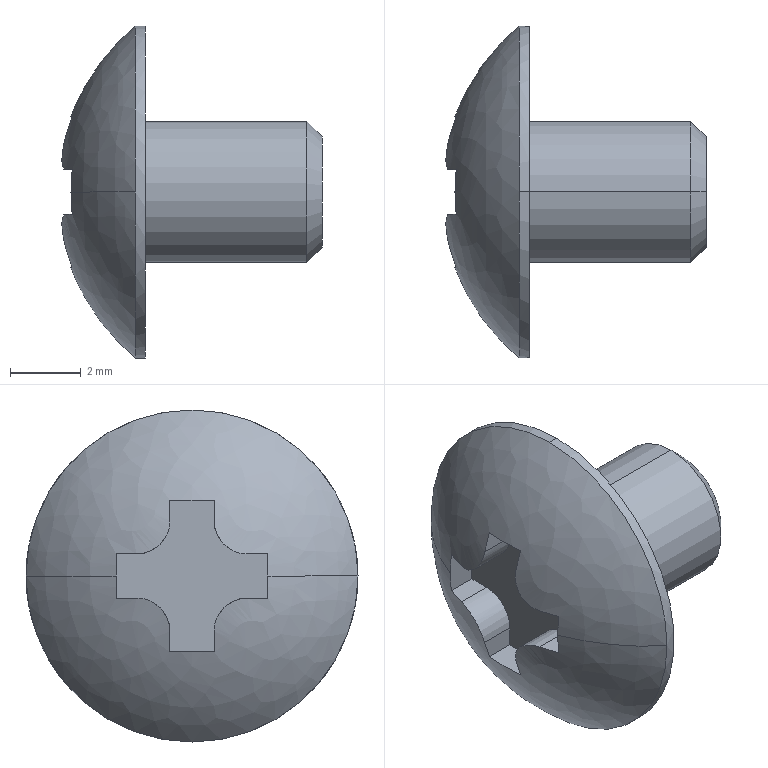Part | STEP file | PN_0001_316_TRSS4-5_Default | 1 solid | 27 faces | box 7.372 x 9.4 x 9.4 mm | volume 153.282 mm3 | plane 15 | cylinder 8 | spline 2 | cone 2 | commonest cylinder face diameters 1.88 x4 4 x2 9.4 x2